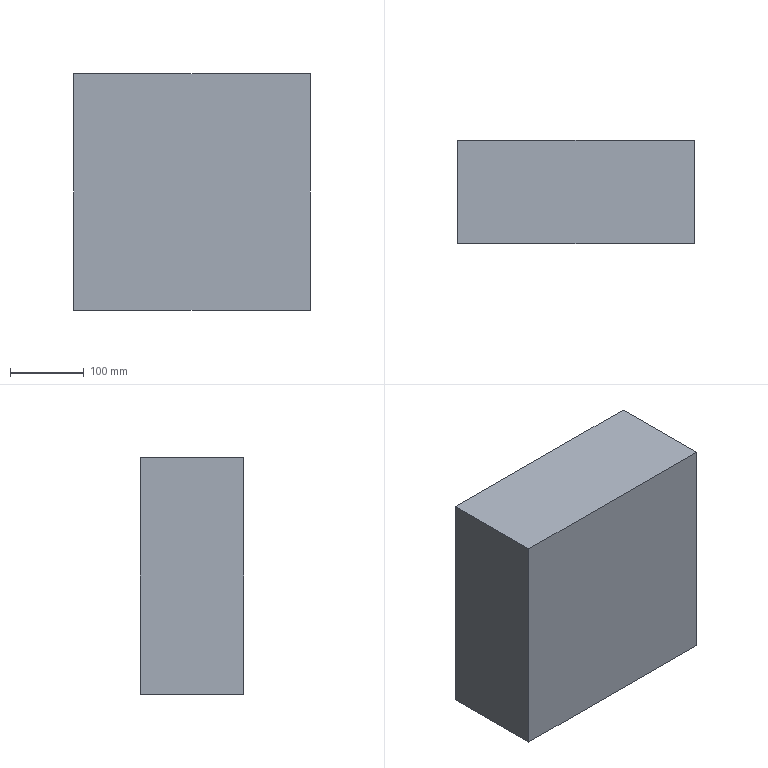Part | NX | features BREP 1 | 1 solid | 6 faces | box 320 x 140 x 320 mm | volume 14336000 mm3 | plane 6
STEP:
#1=CARTESIAN_POINT('',(160.,0.,160.));
#2=VERTEX_POINT('',#1);
#3=CARTESIAN_POINT('',(160.,0.,-160.));
#4=VERTEX_POINT('',#3);
#5=CARTESIAN_POINT('',(160.,0.,-160.));
#6=DIRECTION('',(0.,0.,-1.));
#7=VECTOR('',#6,1000.);
#8=LINE('',#5,#7);
#9=EDGE_CURVE('',#2,#4,#8,.T.);
#10=ORIENTED_EDGE('',*,*,#9,.T.);
#11=CARTESIAN_POINT('',(160.,140.,-160.));
#12=VERTEX_POINT('',#11);
#13=CARTESIAN_POINT('',(160.,140.,-160.));
#14=DIRECTION('',(0.,-1.,0.));
#15=VECTOR('',#14,1000.);
#16=LINE('',#13,#15);
#17=EDGE_CURVE('',#12,#4,#16,.T.);
#18=ORIENTED_EDGE('',*,*,#17,.F.);
#19=CARTESIAN_POINT('',(160.,140.,160.));
#20=VERTEX_POINT('',#19);
#21=CARTESIAN_POINT('',(160.,140.,-160.));
#22=DIRECTION('',(0.,0.,-1.));
#23=VECTOR('',#22,1000.);
#24=LINE('',#21,#23);
#25=EDGE_CURVE('',#20,#12,#24,.T.);
#26=ORIENTED_EDGE('',*,*,#25,.F.);
#27=CARTESIAN_POINT('',(160.,140.,160.));
#28=DIRECTION('',(0.,-1.,0.));
#29=VECTOR('',#28,1000.);
#30=LINE('',#27,#29);
#31=EDGE_CURVE('',#20,#2,#30,.T.);
#32=ORIENTED_EDGE('',*,*,#31,.T.);
#33=EDGE_LOOP('',(#10,#18,#26,#32));
#34=FACE_BOUND('',#33,.T.);
#35=CARTESIAN_POINT('',(160.,140.,-160.));
#36=DIRECTION('',(-1.,0.,0.));
#37=DIRECTION('',(0.,0.,1.));
#38=AXIS2_PLACEMENT_3D('',#35,#36,#37);
#39=PLANE('',#38);
#40=ADVANCED_FACE('',(#34),#39,.F.);
#41=CARTESIAN_POINT('',(-160.,0.,-160.));
#42=VERTEX_POINT('',#41);
#43=CARTESIAN_POINT('',(-160.,0.,-160.));
#44=DIRECTION('',(-1.,0.,0.));
#45=VECTOR('',#44,1000.);
#46=LINE('',#43,#45);
#47=EDGE_CURVE('',#4,#42,#46,.T.);
#48=ORIENTED_EDGE('',*,*,#47,.T.);
#49=CARTESIAN_POINT('',(-160.,140.,-160.));
#50=VERTEX_POINT('',#49);
#51=CARTESIAN_POINT('',(-160.,140.,-160.));
#52=DIRECTION('',(0.,-1.,0.));
#53=VECTOR('',#52,1000.);
#54=LINE('',#51,#53);
#55=EDGE_CURVE('',#50,#42,#54,.T.);
#56=ORIENTED_EDGE('',*,*,#55,.F.);
#57=CARTESIAN_POINT('',(-160.,140.,-160.));
#58=DIRECTION('',(-1.,0.,0.));
#59=VECTOR('',#58,1000.);
#60=LINE('',#57,#59);
#61=EDGE_CURVE('',#12,#50,#60,.T.);
#62=ORIENTED_EDGE('',*,*,#61,.F.);
#63=ORIENTED_EDGE('',*,*,#17,.T.);
#64=EDGE_LOOP('',(#48,#56,#62,#63));
#65=FACE_BOUND('',#64,.T.);
#66=CARTESIAN_POINT('',(-160.,140.,-160.));
#67=DIRECTION('',(0.,0.,1.));
#68=DIRECTION('',(1.,0.,0.));
#69=AXIS2_PLACEMENT_3D('',#66,#67,#68);
#70=PLANE('',#69);
#71=ADVANCED_FACE('',(#65),#70,.F.);
#72=CARTESIAN_POINT('',(-160.,0.,160.));
#73=VERTEX_POINT('',#72);
#74=CARTESIAN_POINT('',(-160.,0.,-160.));
#75=DIRECTION('',(0.,0.,1.));
#76=VECTOR('',#75,1000.);
#77=LINE('',#74,#76);
#78=EDGE_CURVE('',#42,#73,#77,.T.);
#79=ORIENTED_EDGE('',*,*,#78,.T.);
#80=CARTESIAN_POINT('',(-160.,140.,160.));
#81=VERTEX_POINT('',#80);
#82=CARTESIAN_POINT('',(-160.,140.,160.));
#83=DIRECTION('',(0.,-1.,0.));
#84=VECTOR('',#83,1000.);
#85=LINE('',#82,#84);
#86=EDGE_CURVE('',#81,#73,#85,.T.);
#87=ORIENTED_EDGE('',*,*,#86,.F.);
#88=CARTESIAN_POINT('',(-160.,140.,-160.));
#89=DIRECTION('',(0.,0.,1.));
#90=VECTOR('',#89,1000.);
#91=LINE('',#88,#90);
#92=EDGE_CURVE('',#50,#81,#91,.T.);
#93=ORIENTED_EDGE('',*,*,#92,.F.);
#94=ORIENTED_EDGE('',*,*,#55,.T.);
#95=EDGE_LOOP('',(#79,#87,#93,#94));
#96=FACE_BOUND('',#95,.T.);
#97=CARTESIAN_POINT('',(-160.,140.,-160.));
#98=DIRECTION('',(1.,0.,0.));
#99=DIRECTION('',(0.,0.,-1.));
#100=AXIS2_PLACEMENT_3D('',#97,#98,#99);
#101=PLANE('',#100);
#102=ADVANCED_FACE('',(#96),#101,.F.);
#103=CARTESIAN_POINT('',(-160.,0.,160.));
#104=DIRECTION('',(1.,0.,0.));
#105=VECTOR('',#104,1000.);
#106=LINE('',#103,#105);
#107=EDGE_CURVE('',#73,#2,#106,.T.);
#108=ORIENTED_EDGE('',*,*,#107,.T.);
#109=ORIENTED_EDGE('',*,*,#31,.F.);
#110=CARTESIAN_POINT('',(-160.,140.,160.));
#111=DIRECTION('',(1.,0.,0.));
#112=VECTOR('',#111,1000.);
#113=LINE('',#110,#112);
#114=EDGE_CURVE('',#81,#20,#113,.T.);
#115=ORIENTED_EDGE('',*,*,#114,.F.);
#116=ORIENTED_EDGE('',*,*,#86,.T.);
#117=EDGE_LOOP('',(#108,#109,#115,#116));
#118=FACE_BOUND('',#117,.T.);
#119=CARTESIAN_POINT('',(-160.,140.,160.));
#120=DIRECTION('',(0.,0.,-1.));
#121=DIRECTION('',(-1.,0.,0.));
#122=AXIS2_PLACEMENT_3D('',#119,#120,#121);
#123=PLANE('',#122);
#124=ADVANCED_FACE('',(#118),#123,.F.);
#125=ORIENTED_EDGE('',*,*,#25,.T.);
#126=ORIENTED_EDGE('',*,*,#61,.T.);
#127=ORIENTED_EDGE('',*,*,#92,.T.);
#128=ORIENTED_EDGE('',*,*,#114,.T.);
#129=EDGE_LOOP('',(#125,#126,#127,#128));
#130=FACE_BOUND('',#129,.T.);
#131=CARTESIAN_POINT('',(0.,140.,0.));
#132=DIRECTION('',(0.,1.,0.));
#133=DIRECTION('',(0.,0.,1.));
#134=AXIS2_PLACEMENT_3D('',#131,#132,#133);
#135=PLANE('',#134);
#136=ADVANCED_FACE('',(#130),#135,.T.);
#137=ORIENTED_EDGE('',*,*,#9,.F.);
#138=ORIENTED_EDGE('',*,*,#107,.F.);
#139=ORIENTED_EDGE('',*,*,#78,.F.);
#140=ORIENTED_EDGE('',*,*,#47,.F.);
#141=EDGE_LOOP('',(#137,#138,#139,#140));
#142=FACE_BOUND('',#141,.T.);
#143=CARTESIAN_POINT('',(0.,0.,0.));
#144=DIRECTION('',(0.,1.,0.));
#145=DIRECTION('',(0.,0.,1.));
#146=AXIS2_PLACEMENT_3D('',#143,#144,#145);
#147=PLANE('',#146);
#148=ADVANCED_FACE('',(#142),#147,.F.);
#149=CLOSED_SHELL('',(#40,#71,#102,#124,#136,#148));
#150=MANIFOLD_SOLID_BREP('',#149);
#151=(LENGTH_UNIT()NAMED_UNIT(*)SI_UNIT(.MILLI.,.METRE.));
#152=UNCERTAINTY_MEASURE_WITH_UNIT(LENGTH_MEASURE(0.00001),#151,'','');
#153=(NAMED_UNIT(*)PLANE_ANGLE_UNIT()SI_UNIT($,.RADIAN.));
#154=(NAMED_UNIT(*)SI_UNIT($,.STERADIAN.)SOLID_ANGLE_UNIT());
#155=(GEOMETRIC_REPRESENTATION_CONTEXT(3)GLOBAL_UNCERTAINTY_ASSIGNED_CONTEXT((#152))GLOBAL_UNIT_ASSIGNED_CONTEXT((#151,#153,#154))REPRESENTATION_CONTEXT('',''));
#156=ADVANCED_BREP_SHAPE_REPRESENTATION('',(#150),#155);